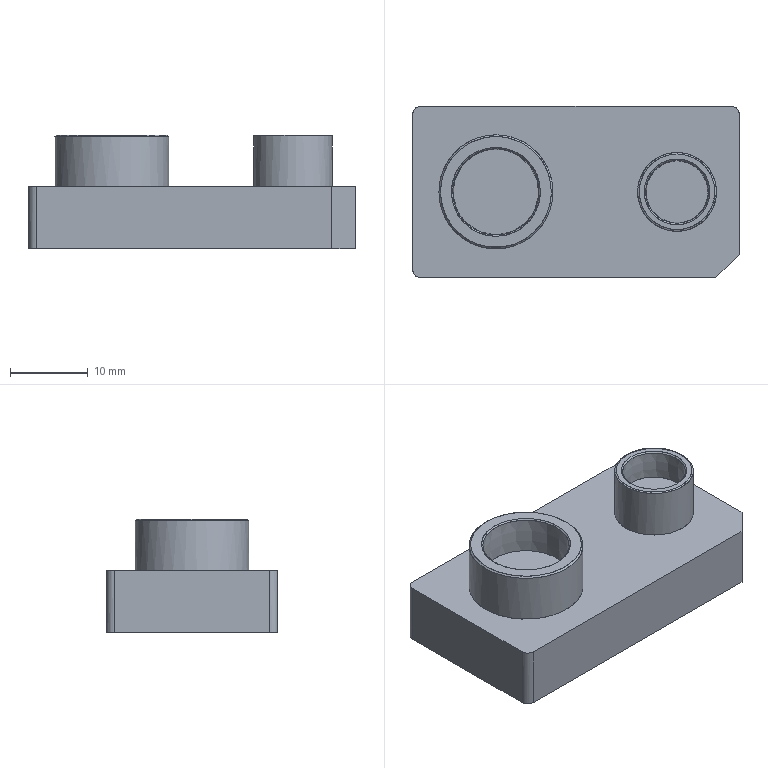NC program | PowerMill | posted by the shop | part box 42 x 22 x 14.621 mm
Lines 14234 to 15750 of 126517:
( TOOL ID   D4_2 )
( TOOL DIA. 4. TIP RAD 0 LENGTH 61.8 )
( Z = -6.79 )
T14 M6
T13
G91 G28 Z0
G0 G90 G54
M08
S18000 M3
X0 Y0 M8
G43 Z10.801 H14
X-9.103 Y-9.671
Z.911
G1 Z-.289 F1200
X-9.107 Y-9.621 F2000
X-9.116 Y-9.571
X-9.128 Y-9.522
X-9.144 Y-9.474
X-9.164 Y-9.428
X-9.187 Y-9.383
X-9.214 Y-9.34
X-9.244 Y-9.3
X-9.278 Y-9.262
X-9.314 Y-9.226
X-9.353 Y-9.194
X-9.394 Y-9.165
X-9.437 Y-9.139
X-9.483 Y-9.117
X-9.53 Y-9.098
X-9.578 Y-9.083
X-9.627 Y-9.072
X-9.677 Y-9.065
X-9.728 Y-9.062
X-9.773 Y-9.063
X-9.966 Y-9.072
X-10.153 Y-9.077
X-10.341 Y-9.078
X-10.531 Y-9.075
X-10.721 Y-9.069
X-10.911 Y-9.058
X-11.101 Y-9.043
X-11.292 Y-9.024
X-11.478 Y-9.002
X-11.665 Y-8.976
X-11.851 Y-8.945
X-12.039 Y-8.911
X-12.225 Y-8.873
X-12.412 Y-8.83
X-12.597 Y-8.784
X-12.781 Y-8.734
X-12.963 Y-8.68
X-13.139 Y-8.624
X-13.315 Y-8.564
X-13.493 Y-8.5
X-13.671 Y-8.431
X-13.847 Y-8.358
X-14.02 Y-8.283
X-14.188 Y-8.206
X-14.351 Y-8.126
X-14.519 Y-8.041
X-14.668 Y-7.961
X-14.833 Y-7.868
X-14.997 Y-7.771
X-15.158 Y-7.671
X-15.318 Y-7.568
X-15.469 Y-7.465
X-15.595 Y-7.377
X-15.719 Y-7.287
X-15.841 Y-7.195
X-15.961 Y-7.1
X-16.064 Y-7.017
X-16.166 Y-6.932
X-16.266 Y-6.846
X-16.365 Y-6.758
X-16.509 Y-6.627
X-16.618 Y-6.523
X-16.726 Y-6.417
X-16.832 Y-6.309
X-16.955 Y-6.179
X-17.057 Y-6.067
X-17.158 Y-5.954
X-17.256 Y-5.839
X-17.352 Y-5.723
X-17.472 Y-5.571
X-17.588 Y-5.418
X-17.701 Y-5.264
X-17.809 Y-5.108
X-17.914 Y-4.951
X-18.015 Y-4.792
X-18.113 Y-4.629
X-18.209 Y-4.464
X-18.301 Y-4.297
X-18.39 Y-4.127
X-18.476 Y-3.955
X-18.553 Y-3.791
X-18.627 Y-3.625
X-18.698 Y-3.458
X-18.768 Y-3.283
X-18.836 Y-3.103
X-18.899 Y-2.924
X-18.956 Y-2.751
X-19.009 Y-2.577
X-19.055 Y-2.416
X-19.098 Y-2.254
X-19.138 Y-2.091
X-19.176 Y-1.927
X-19.213 Y-1.748
X-19.246 Y-1.568
X-19.276 Y-1.388
X-19.302 Y-1.207
X-19.324 Y-1.026
X-19.344 Y-.837
X-19.359 Y-.649
X-19.371 Y-.46
X-19.378 Y-.285
X-19.382 Y-.11
Y.065
X-19.379 Y.24
X-19.373 Y.427
X-19.362 Y.616
X-19.347 Y.807
X-19.328 Y.997
X-19.305 Y1.185
X-19.279 Y1.37
X-19.248 Y1.556
X-19.214 Y1.742
X-19.175 Y1.929
X-19.132 Y2.116
X-19.087 Y2.3
X-19.038 Y2.479
X-18.985 Y2.658
X-18.928 Y2.837
X-18.866 Y3.018
X-18.8 Y3.198
X-18.731 Y3.377
X-18.659 Y3.552
X-18.584 Y3.724
X-18.505 Y3.894
X-18.423 Y4.063
X-18.336 Y4.231
X-18.246 Y4.398
X-18.152 Y4.564
X-18.053 Y4.729
X-17.951 Y4.892
X-17.848 Y5.05
X-17.741 Y5.206
X-17.631 Y5.361
X-17.517 Y5.513
X-17.399 Y5.664
X-17.278 Y5.812
X-17.174 Y5.936
X-17.067 Y6.057
X-16.957 Y6.176
X-16.839 Y6.301
X-16.726 Y6.417
X-16.611 Y6.53
X-16.494 Y6.641
X-16.361 Y6.762
X-16.246 Y6.864
X-16.129 Y6.963
X-16.011 Y7.06
X-15.891 Y7.156
X-15.753 Y7.261
X-15.61 Y7.367
X-15.457 Y7.474
X-15.299 Y7.58
X-15.148 Y7.678
X-15.001 Y7.769
X-14.846 Y7.861
X-14.689 Y7.949
X-14.526 Y8.037
X-14.355 Y8.124
X-14.189 Y8.205
X-14.026 Y8.28
X-13.861 Y8.353
X-13.695 Y8.421
X-13.519 Y8.49
X-13.341 Y8.555
X-13.162 Y8.617
X-12.982 Y8.674
X-12.801 Y8.728
X-12.62 Y8.778
X-12.438 Y8.824
X-12.252 Y8.867
X-12.066 Y8.906
X-11.879 Y8.941
X-11.692 Y8.972
X-11.505 Y8.999
X-11.317 Y9.022
X-11.127 Y9.041
X-10.936 Y9.056
X-10.746 Y9.067
X-10.555 Y9.075
X-10.365 Y9.078
X-10.174 Y9.077
X-9.984 Y9.073
X-9.794 Y9.064
X-9.604 Y9.051
X-9.414 Y9.034
X-9.225 Y9.014
X-9.036 Y8.989
X-8.847 Y8.96
X-8.659 Y8.928
X-8.473 Y8.892
X-8.288 Y8.851
X-8.103 Y8.807
X-7.919 Y8.759
X-7.735 Y8.707
X-7.552 Y8.651
X-7.377 Y8.593
X-7.203 Y8.532
X-7.026 Y8.465
X-6.865 Y8.401
X-6.706 Y8.334
X-6.542 Y8.262
X-6.385 Y8.189
X-6.23 Y8.112
X-6.072 Y8.031
X-5.916 Y7.947
X-5.761 Y7.86
X-5.609 Y7.77
X-5.458 Y7.676
X-5.311 Y7.581
X-5.171 Y7.487
X-5.033 Y7.391
X-4.898 Y7.293
X-4.764 Y7.191
X-4.634 Y7.09
X-4.506 Y6.985
X-4.369 Y6.869
X-4.237 Y6.752
X-4.106 Y6.633
X-3.978 Y6.511
X-3.853 Y6.387
X-3.73 Y6.26
X-3.617 Y6.139
X-3.505 Y6.015
X-3.396 Y5.889
X-3.289 Y5.762
X-3.185 Y5.633
X-3.084 Y5.502
X-2.985 Y5.37
X-2.888 Y5.236
X-2.794 Y5.1
X-2.702 Y4.962
X-2.6 Y4.801
X-2.502 Y4.64
X-2.408 Y4.479
X-2.318 Y4.316
X-2.229 Y4.147
X-2.144 Y3.978
X-2.064 Y3.808
X-1.988 Y3.64
X-1.917 Y3.474
X-1.846 Y3.296
X-1.778 Y3.118
X-1.715 Y2.938
X-1.655 Y2.757
X-1.599 Y2.575
X-1.551 Y2.406
X-1.506 Y2.235
X-1.464 Y2.064
X-1.423 Y1.877
X-1.388 Y1.705
X-1.356 Y1.531
X-1.328 Y1.357
X-1.302 Y1.168
X-1.279 Y.978
X-1.261 Y.787
X-1.246 Y.597
X-1.235 Y.406
X-1.229 Y.215
X-1.226 Y.024
X-1.228 Y-.167
X-1.233 Y-.352
X-1.242 Y-.538
X-1.255 Y-.727
X-1.273 Y-.918
X-1.294 Y-1.107
X-1.319 Y-1.292
X-1.347 Y-1.476
X-1.379 Y-1.66
X-1.416 Y-1.845
X-1.456 Y-2.031
X-1.501 Y-2.217
X-1.549 Y-2.399
X-1.601 Y-2.58
X-1.653 Y-2.752
X-1.709 Y-2.923
X-1.769 Y-3.093
X-1.832 Y-3.261
X-1.899 Y-3.428
X-1.968 Y-3.595
X-2.045 Y-3.768
X-2.121 Y-3.931
X-2.201 Y-4.092
X-2.283 Y-4.251
X-2.372 Y-4.415
X-2.468 Y-4.582
X-2.561 Y-4.739
X-2.656 Y-4.891
X-2.75 Y-5.035
X-2.846 Y-5.176
X-2.946 Y-5.316
X-3.047 Y-5.454
X-3.151 Y-5.59
X-3.258 Y-5.724
X-3.381 Y-5.872
X-3.507 Y-6.018
X-3.636 Y-6.16
X-3.768 Y-6.3
X-3.902 Y-6.436
X-4.026 Y-6.557
X-4.153 Y-6.676
X-4.285 Y-6.795
X-4.416 Y-6.909
X-4.549 Y-7.021
X-4.685 Y-7.13
X-4.83 Y-7.242
X-4.978 Y-7.352
X-5.129 Y-7.459
X-5.282 Y-7.562
X-5.436 Y-7.662
X-5.588 Y-7.757
X-5.742 Y-7.849
X-5.898 Y-7.937
X-6.056 Y-8.022
X-6.215 Y-8.105
X-6.376 Y-8.184
X-6.549 Y-8.265
X-6.699 Y-8.332
X-6.851 Y-8.396
X-7.004 Y-8.457
X-7.158 Y-8.515
X-7.313 Y-8.571
X-7.469 Y-8.624
X-7.644 Y-8.679
X-7.82 Y-8.732
X-7.999 Y-8.781
X-8.179 Y-8.826
X-8.358 Y-8.867
X-8.538 Y-8.905
X-8.719 Y-8.938
X-8.907 Y-8.97
X-9.095 Y-8.997
X-9.284 Y-9.021
X-9.472 Y-9.04
X-9.658 Y-9.055
X-9.773 Y-9.063
X-9.823 Y-9.068
X-9.873 Y-9.077
X-9.921 Y-9.09
X-9.969 Y-9.107
X-10.015 Y-9.128
X-10.06 Y-9.152
X-10.102 Y-9.179
X-10.142 Y-9.21
X-10.179 Y-9.244
X-10.214 Y-9.281
X-10.246 Y-9.32
X-10.274 Y-9.362
X-10.299 Y-9.406
X-10.321 Y-9.451
X-10.339 Y-9.499
X-10.353 Y-9.547
X-10.363 Y-9.597
X-10.369 Y-9.647
X-10.372 Y-9.697
X-10.37 Y-9.742
X-9.096 Y-9.684 Z-.309
X-9.101 Y-9.634
X-9.11 Y-9.584
X-9.122 Y-9.535
X-9.139 Y-9.488
X-9.159 Y-9.441
X-9.183 Y-9.397
X-9.21 Y-9.354
X-9.241 Y-9.314
X-9.275 Y-9.276
X-9.311 Y-9.241
X-9.35 Y-9.209
X-9.392 Y-9.181
X-9.436 Y-9.155
X-9.481 Y-9.133
X-9.528 Y-9.115
X-9.577 Y-9.101
X-9.626 Y-9.09
X-9.676 Y-9.084
X-9.727 Y-9.081
X-9.772 Y-9.082
X-9.88 Y-9.088
X-10.069 Y-9.095
X-10.258 Y-9.098
X-10.448 Y-9.097
X-10.638 Y-9.092
X-10.827 Y-9.083
X-11.017 Y-9.07
X-11.206 Y-9.053
X-11.396 Y-9.032
X-11.585 Y-9.008
X-11.774 Y-8.979
X-11.958 Y-8.947
X-12.143 Y-8.91
X-12.329 Y-8.87
X-12.516 Y-8.825
X-12.696 Y-8.778
X-12.877 Y-8.727
X-13.058 Y-8.671
X-13.241 Y-8.611
X-13.412 Y-8.551
X-13.582 Y-8.488
X-13.754 Y-8.419
X-13.929 Y-8.345
X-14.102 Y-8.267
X-14.274 Y-8.187
X-14.444 Y-8.102
X-14.612 Y-8.014
X-14.778 Y-7.922
X-14.943 Y-7.827
X-15.105 Y-7.728
X-15.266 Y-7.626
X-15.425 Y-7.52
X-15.574 Y-7.416
X-15.722 Y-7.309
X-15.867 Y-7.2
X-16.01 Y-7.087
X-16.151 Y-6.971
X-16.271 Y-6.869
X-16.387 Y-6.766
X-16.508 Y-6.655
X-16.624 Y-6.546
X-16.737 Y-6.434
X-16.848 Y-6.321
X-16.976 Y-6.186
X-17.083 Y-6.069
X-17.188 Y-5.949
X-17.291 Y-5.828
X-17.41 Y-5.682
X-17.512 Y-5.552
X-17.611 Y-5.421
X-17.709 Y-5.287
X-17.803 Y-5.152
X-17.895 Y-5.015
X-17.985 Y-4.877
X-18.082 Y-4.721
X-18.177 Y-4.561
X-18.269 Y-4.398
X-18.359 Y-4.231
X-18.446 Y-4.06
X-18.531 Y-3.885
X-18.608 Y-3.719
X-18.681 Y-3.55
X-18.753 Y-3.377
X-18.822 Y-3.199
X-18.887 Y-3.019
X-18.948 Y-2.841
X-19.004 Y-2.665
X-19.056 Y-2.489
X-19.104 Y-2.311
X-19.151 Y-2.126
X-19.193 Y-1.94
X-19.232 Y-1.754
X-19.267 Y-1.567
X-19.297 Y-1.38
X-19.324 Y-1.192
X-19.347 Y-1.004
X-19.366 Y-.815
X-19.381 Y-.626
X-19.392 Y-.436
X-19.399 Y-.246
X-19.402 Y-.055
Y.136
X-19.397 Y.326
X-19.388 Y.516
X-19.375 Y.706
X-19.358 Y.895
X-19.338 Y1.083
X-19.313 Y1.273
X-19.284 Y1.461
X-19.252 Y1.648
X-19.216 Y1.835
X-19.175 Y2.02
X-19.131 Y2.205
X-19.084 Y2.388
X-19.032 Y2.571
X-18.976 Y2.753
X-18.917 Y2.933
X-18.854 Y3.111
X-18.788 Y3.288
X-18.727 Y3.44
X-18.664 Y3.592
X-18.598 Y3.742
X-18.529 Y3.89
X-18.457 Y4.038
X-18.379 Y4.193
X-18.298 Y4.346
X-18.214 Y4.497
X-18.126 Y4.647
X-18.036 Y4.795
X-17.95 Y4.931
X-17.862 Y5.065
X-17.771 Y5.199
X-17.678 Y5.33
X-17.583 Y5.459
X-17.485 Y5.587
X-17.385 Y5.713
X-17.273 Y5.85
X-17.157 Y5.985
X-17.035 Y6.122
X-16.905 Y6.261
X-16.773 Y6.398
X-16.645 Y6.525
X-16.526 Y6.638
X-16.439 Y6.718
X-16.352 Y6.797
X-16.264 Y6.875
X-16.15 Y6.972
X-16.034 Y7.067
X-15.917 Y7.16
X-15.799 Y7.252
X-15.679 Y7.341
X-15.529 Y7.448
X-15.376 Y7.553
X-15.216 Y7.658
X-15.053 Y7.76
X-14.894 Y7.856
X-14.735 Y7.947
X-14.573 Y8.035
X-14.407 Y8.121
X-14.237 Y8.204
X-14.064 Y8.285
X-13.889 Y8.362
X-13.716 Y8.434
X-13.548 Y8.5
X-13.379 Y8.563
X-13.209 Y8.622
X-13.036 Y8.679
X-12.864 Y8.731
X-12.69 Y8.78
X-12.516 Y8.825
X-12.331 Y8.87
X-12.151 Y8.909
X-11.97 Y8.944
X-11.783 Y8.977
X-11.595 Y9.006
X-11.405 Y9.031
X-11.214 Y9.052
X-11.025 Y9.07
X-10.836 Y9.083
X-10.647 Y9.092
X-10.458 Y9.097
X-10.274 Y9.098
X-10.089 Y9.095
X-9.905 Y9.089
X-9.72 Y9.079
X-9.533 Y9.066
X-9.349 Y9.048
X-9.166 Y9.027
X-8.983 Y9.002
X-8.794 Y8.972
X-8.606 Y8.938
X-8.42 Y8.901
X-8.236 Y8.86
X-8.054 Y8.815
X-7.868 Y8.766
X-7.684 Y8.713
X-7.502 Y8.656
X-7.321 Y8.595
X-7.141 Y8.531
X-6.964 Y8.463
X-6.788 Y8.391
X-6.613 Y8.316
X-6.44 Y8.237
X-6.268 Y8.154
X-6.099 Y8.068
X-5.931 Y7.978
X-5.772 Y7.889
X-5.661 Y7.824
X-5.55 Y7.757
X-5.441 Y7.689
X-5.332 Y7.619
X-5.224 Y7.548
X-5.073 Y7.443
X-4.923 Y7.336
X-4.775 Y7.225
X-4.63 Y7.112
X-4.487 Y6.995
X-4.347 Y6.876
X-4.205 Y6.75
X-4.064 Y6.621
X-3.926 Y6.488
X-3.792 Y6.354
X-3.661 Y6.217
X-3.534 Y6.078
X-3.415 Y5.942
X-3.298 Y5.804
X-3.184 Y5.664
X-3.073 Y5.522
X-2.965 Y5.377
X-2.868 Y5.242
X-2.773 Y5.105
X-2.681 Y4.967
X-2.578 Y4.805
X-2.482 Y4.647
X-2.391 Y4.49
X-2.298 Y4.322
X-2.21 Y4.153
X-2.126 Y3.985
X-2.045 Y3.816
X-1.967 Y3.641
X-1.892 Y3.466
X-1.822 Y3.289
X-1.755 Y3.111
X-1.692 Y2.932
X-1.632 Y2.752
X-1.577 Y2.57
X-1.525 Y2.387
X-1.477 Y2.203
X-1.433 Y2.018
X-1.393 Y1.832
X-1.356 Y1.646
X-1.324 Y1.459
X-1.295 Y1.271
X-1.271 Y1.082
X-1.25 Y.895
X-1.234 Y.707
X-1.221 Y.519
X-1.212 Y.33
X-1.207 Y.141
X-1.206 Y-.049
X-1.209 Y-.238
X-1.216 Y-.427
X-1.227 Y-.617
X-1.242 Y-.807
X-1.261 Y-.997
X-1.284 Y-1.187
X-1.311 Y-1.376
X-1.341 Y-1.562
X-1.376 Y-1.749
X-1.414 Y-1.935
X-1.457 Y-2.122
X-1.504 Y-2.308
X-1.551 Y-2.482
X-1.6 Y-2.649
X-1.653 Y-2.814
X-1.709 Y-2.983
X-1.771 Y-3.155
X-1.833 Y-3.318
X-1.897 Y-3.479
X-1.966 Y-3.638
X-2.044 Y-3.813
X-2.122 Y-3.977
X-2.203 Y-4.141
X-2.292 Y-4.31
X-2.384 Y-4.477
X-2.48 Y-4.642
X-2.578 Y-4.805
X-2.68 Y-4.965
X-2.785 Y-5.122
X-2.89 Y-5.273
X-2.998 Y-5.422
X-3.109 Y-5.568
X-3.223 Y-5.712
X-3.34 Y-5.854
X-3.459 Y-5.993
X-3.585 Y-6.134
X-3.714 Y-6.272
X-3.846 Y-6.408
X-3.982 Y-6.542
X-4.12 Y-6.673
X-4.26 Y-6.8
X-4.403 Y-6.925
X-4.547 Y-7.045
X-4.693 Y-7.162
X-4.843 Y-7.276
X-4.996 Y-7.389
X-5.152 Y-7.498
X-5.312 Y-7.606
X-5.473 Y-7.709
X-5.636 Y-7.809
X-5.787 Y-7.898
X-5.94 Y-7.983
X-6.095 Y-8.066
X-6.259 Y-8.149
X-6.416 Y-8.225
X-6.575 Y-8.299
X-6.736 Y-8.369
X-6.904 Y-8.439
X-7.074 Y-8.505
X-7.253 Y-8.571
X-7.426 Y-8.631
X-7.599 Y-8.687
X-7.774 Y-8.739
X-7.959 Y-8.791
X-8.144 Y-8.838
X-8.328 Y-8.881
X-8.512 Y-8.92
X-8.693 Y-8.954
X-8.874 Y-8.985
X-9.062 Y-9.013
X-9.245 Y-9.036
X-9.428 Y-9.056
X-9.498 Y-9.062
X-9.689 Y-9.077
X-9.772 Y-9.082
X-9.822 Y-9.087
X-9.872 Y-9.096
X-9.921 Y-9.108
X-9.968 Y-9.125
X-10.015 Y-9.145
X-10.059 Y-9.169
X-10.102 Y-9.196
X-10.142 Y-9.227
X-10.18 Y-9.261
X-10.215 Y-9.297
X-10.246 Y-9.336
X-10.275 Y-9.378
X-10.301 Y-9.422
X-10.322 Y-9.467
X-10.341 Y-9.514
X-10.355 Y-9.563
X-10.366 Y-9.612
X-10.372 Y-9.662
X-10.375 Y-9.713
X-10.374 Y-9.758
X-9.094 Y-9.704 Z-.329
X-9.099 Y-9.653
X-9.108 Y-9.604
X-9.121 Y-9.555
X-9.137 Y-9.507
X-9.158 Y-9.461
X-9.182 Y-9.416
X-9.209 Y-9.374
X-9.24 Y-9.333
X-9.273 Y-9.296
X-9.31 Y-9.261
X-9.349 Y-9.229
X-9.391 Y-9.2
X-9.434 Y-9.175
X-9.48 Y-9.153
X-9.527 Y-9.135
X-9.576 Y-9.121
X-9.625 Y-9.11
X-9.675 Y-9.104
X-9.725 Y-9.101
X-9.77 Y-9.102
X-9.869 Y-9.108
X-10.06 Y-9.115
X-10.251 Y-9.118
X-10.441 Y-9.117
X-10.631 Y-9.112
X-10.821 Y-9.104
X-11.009 Y-9.091
X-11.198 Y-9.074
X-11.387 Y-9.053
X-11.576 Y-9.029
X-11.764 Y-9.
X-11.951 Y-8.968
X-12.138 Y-8.932
X-12.324 Y-8.892
X-12.508 Y-8.848
X-12.684 Y-8.802
X-12.859 Y-8.753
X-13.033 Y-8.7
X-13.215 Y-8.641
X-13.391 Y-8.58
X-13.562 Y-8.517
X-13.731 Y-8.45
X-13.898 Y-8.38
X-14.074 Y-8.302
X-14.247 Y-8.221
X-14.419 Y-8.137
X-14.589 Y-8.049
X-14.756 Y-7.958
X-14.921 Y-7.863
X-15.084 Y-7.765
X-15.242 Y-7.665
X-15.401 Y-7.561
X-15.559 Y-7.451
X-15.714 Y-7.34
X-15.867 Y-7.225
X-16.016 Y-7.108
X-16.163 Y-6.987
X-16.301 Y-6.869
X-16.434 Y-6.75
X-16.573 Y-6.621
X-16.709 Y-6.49
X-16.843 Y-6.355
X-16.975 Y-6.216
X-17.102 Y-6.078
X-17.225 Y-5.937
X-17.346 Y-5.793
X-17.464 Y-5.646
X-17.583 Y-5.492
X-17.695 Y-5.341
X-17.8 Y-5.192
X-17.894 Y-5.054
X-18.003 Y-4.885
X-18.1 Y-4.73
X-18.186 Y-4.585
X-18.26 Y-4.455
X-18.333 Y-4.324
X-18.402 Y-4.192
X-18.469 Y-4.058
X-18.535 Y-3.923
X-18.611 Y-3.761
X-18.685 Y-3.593
X-18.755 Y-3.424
X-18.821 Y-3.258
X-18.888 Y-3.076
X-18.951 Y-2.895
X-19.009 Y-2.714
X-19.064 Y-2.533
X-19.114 Y-2.351
X-19.162 Y-2.166
X-19.205 Y-1.98
X-19.244 Y-1.794
X-19.28 Y-1.607
X-19.311 Y-1.42
X-19.338 Y-1.24
X-19.361 Y-1.059
X-19.38 Y-.878
X-19.396 Y-.695
X-19.408 Y-.514
X-19.416 Y-.332
X-19.421 Y-.149
X-19.422 Y.035
X-19.42 Y.219
X-19.414 Y.406
X-19.404 Y.591
X-19.39 Y.774
X-19.372 Y.957
X-19.351 Y1.136
X-19.327 Y1.315
X-19.3 Y1.493
X-19.268 Y1.671
X-19.233 Y1.847
X-19.195 Y2.023
X-19.151 Y2.208
X-19.103 Y2.392
X-19.052 Y2.574
X-18.997 Y2.754
X-18.937 Y2.936
X-18.873 Y3.117
X-18.814 Y3.276
X-18.752 Y3.433
X-18.686 Y3.589
X-18.613 Y3.755
X-18.542 Y3.909
X-18.468 Y4.061
X-18.391 Y4.212
X-18.3 Y4.382
X-18.21 Y4.543
X-18.117 Y4.702
X-18.019 Y4.861
X-17.916 Y5.02
X-17.808 Y5.18
X-17.695 Y5.34
X-17.592 Y5.48
X-17.48 Y5.625
X-17.357 Y5.779
X-17.253 Y5.905
X-17.146 Y6.028
X-17.036 Y6.15
X-16.913 Y6.282
X-16.8 Y6.399
X-16.684 Y6.515
X-16.566 Y6.628
X-16.446 Y6.739
X-16.302 Y6.868
X-16.156 Y6.992
X-16.011 Y7.112
X-15.865 Y7.227
X-15.726 Y7.331
X-15.59 Y7.43
X-15.452 Y7.526
X-15.312 Y7.62
X-15.17 Y7.711
X-15.026 Y7.8
X-14.875 Y7.89
X-14.721 Y7.978
X-14.565 Y8.062
X-14.408 Y8.143
X-14.249 Y8.22
X-14.093 Y8.294
X-13.936 Y8.364
X-13.768 Y8.435
X-13.608 Y8.499
X-13.447 Y8.56
X-13.265 Y8.624
X-13.083 Y8.684
X-12.899 Y8.741
X-12.715 Y8.794
X-12.53 Y8.842
X-12.344 Y8.887
X-12.158 Y8.928
X-11.972 Y8.964
X-11.785 Y8.997
X-11.597 Y9.026
X-11.407 Y9.051
X-11.216 Y9.072
X-11.031 Y9.089
X-10.846 Y9.102
X-10.659 Y9.111
X-10.469 Y9.117
X-10.277 Y9.118
X-10.088 Y9.116
X-9.902 Y9.109
X-9.717 Y9.099
X-9.526 Y9.085
X-9.336 Y9.067
X-9.146 Y9.044
X-8.957 Y9.018
X-8.768 Y8.988
X-8.579 Y8.954
X-8.395 Y8.916
X-8.21 Y8.874
X-8.026 Y8.829
X-7.841 Y8.779
X-7.655 Y8.725
X-7.483 Y8.671
X-7.311 Y8.613
X-7.14 Y8.552
X-6.967 Y8.485
X-6.789 Y8.413
X-6.614 Y8.338
X-6.446 Y8.262
X-6.283 Y8.183
X-6.121 Y8.102
X-5.961 Y8.017
X-5.793 Y7.924
X-5.628 Y7.828
X-5.467 Y7.729
X-5.308 Y7.628
X-5.153 Y7.523
X-5. Y7.416
X-4.851 Y7.307
X-4.705 Y7.196
X-4.561 Y7.082
X-4.419 Y6.965
X-4.28 Y6.844
X-4.167 Y6.743
X-4.053 Y6.638
X-3.933 Y6.522
X-3.815 Y6.406
X-3.698 Y6.285
X-3.573 Y6.151
X-3.457 Y6.021
X-3.348 Y5.895
X-3.235 Y5.759
X-3.124 Y5.621
X-3.016 Y5.48
X-2.911 Y5.338
X-2.806 Y5.188
X-2.699 Y5.03
X-2.597 Y4.872
X-2.498 Y4.711
X-2.401 Y4.548
X-2.309 Y4.384
X-2.218 Y4.214
X-2.134 Y4.048
X-2.054 Y3.884
X-1.977 Y3.714
X-1.9 Y3.535
X-1.828 Y3.361
X-1.76 Y3.185
X-1.696 Y3.006
X-1.635 Y2.826
X-1.578 Y2.643
X-1.525 Y2.46
X-1.475 Y2.276
X-1.429 Y2.092
X-1.388 Y1.906
X-1.35 Y1.72
X-1.316 Y1.532
X-1.286 Y1.344
X-1.26 Y1.155
X-1.238 Y.968
X-1.22 Y.781
X-1.206 Y.593
X-1.195 Y.404
X-1.189 Y.214
X-1.186 Y.025
X-1.188 Y-.164
X-1.193 Y-.353
X-1.202 Y-.543
X-1.216 Y-.733
X-1.233 Y-.923
X-1.254 Y-1.113
X-1.28 Y-1.302
X-1.309 Y-1.49
X-1.342 Y-1.677
X-1.379 Y-1.864
X-1.42 Y-2.051
X-1.465 Y-2.236
X-1.514 Y-2.421
X-1.566 Y-2.605
X-1.622 Y-2.786
X-1.682 Y-2.967
X-1.746 Y-3.146
X-1.813 Y-3.323
X-1.884 Y-3.499
X-1.959 Y-3.674
X-2.038 Y-3.848
X-2.115 Y-4.008
X-2.194 Y-4.166
X-2.276 Y-4.323
X-2.362 Y-4.479
X-2.45 Y-4.632
X-2.542 Y-4.784
X-2.637 Y-4.933
X-2.743 Y-5.095
X-2.85 Y-5.251
X-2.944 Y-5.383
X-3.041 Y-5.512
X-3.14 Y-5.64
X-3.247 Y-5.773
X-3.35 Y-5.897
X-3.455 Y-6.019
X-3.549 Y-6.124
X-3.645 Y-6.228
X-3.742 Y-6.33
X-3.84 Y-6.431
X-3.941 Y-6.53
X-4.059 Y-6.643
X-4.178 Y-6.754
X-4.3 Y-6.862
X-4.424 Y-6.968
X-4.549 Y-7.072
X-4.697 Y-7.19
X-4.847 Y-7.305
X-5.001 Y-7.417
X-5.158 Y-7.527
X-5.314 Y-7.631
X-5.474 Y-7.733
X-5.636 Y-7.832
X-5.802 Y-7.929
X-5.971 Y-8.022
X-6.137 Y-8.11
X-6.305 Y-8.194
X-6.475 Y-8.275
X-6.649 Y-8.353
X-6.822 Y-8.427
X-6.997 Y-8.497
X-7.174 Y-8.564
X-7.352 Y-8.627
X-7.532 Y-8.686
X-7.718 Y-8.743
X-7.904 Y-8.796
X-8.088 Y-8.845
X-8.272 Y-8.889
X-8.456 Y-8.929
X-8.625 Y-8.962
X-8.795 Y-8.992
X-8.965 Y-9.019
X-9.136 Y-9.043
X-9.298 Y-9.062
X-9.488 Y-9.081
X-9.679 Y-9.097
X-9.77 Y-9.102
X-9.821 Y-9.107
X-9.87 Y-9.116
X-9.919 Y-9.129
X-9.967 Y-9.145
X-10.013 Y-9.166
X-10.058 Y-9.189
X-10.1 Y-9.217
X-10.141 Y-9.247
X-10.178 Y-9.281
X-10.213 Y-9.318
X-10.245 Y-9.357
X-10.274 Y-9.398
X-10.299 Y-9.442
X-10.321 Y-9.488
X-10.339 Y-9.535
X-10.353 Y-9.583
X-10.364 Y-9.633
X-10.37 Y-9.683
X-10.373 Y-9.733
X-10.372 Y-9.778
X-9.092 Y-9.723 Z-.349
X-9.097 Y-9.672
X-9.106 Y-9.623
X-9.119 Y-9.574
X-9.136 Y-9.526
X-9.156 Y-9.48
X-9.18 Y-9.435
X-9.208 Y-9.393
X-9.238 Y-9.353
X-9.272 Y-9.315
X-9.308 Y-9.28
X-9.348 Y-9.248
X-9.389 Y-9.22
X-9.433 Y-9.194
X-9.479 Y-9.173
X-9.526 Y-9.155
X-9.574 Y-9.14
X-9.624 Y-9.13
X-9.674 Y-9.123
X-9.724 Y-9.121
X-9.769 Y-9.122
X-9.858 Y-9.127
X-10.038 Y-9.134
X-10.219 Y-9.138
X-10.399
X-10.579 Y-9.134
X-10.765 Y-9.127
X-10.945 Y-9.116
X-11.124 Y-9.101
X-11.316 Y-9.082
X-11.506 Y-9.059
X-11.696 Y-9.032
X-11.885 Y-9.
X-12.073 Y-8.965
X-12.258 Y-8.927
X-12.442 Y-8.885
X-12.626 Y-8.838
X-12.81 Y-8.788
X-12.994 Y-8.733
X-13.177 Y-8.675
X-13.358 Y-8.613
X-13.538 Y-8.547
X-13.716 Y-8.478
X-13.887 Y-8.407
X-14.058 Y-8.332
X-14.23 Y-8.252
X-14.402 Y-8.168
X-14.573 Y-8.08
X-14.741 Y-7.989
X-14.906 Y-7.895
X-15.066 Y-7.8
X-15.223 Y-7.701
X-15.375 Y-7.602
X-15.524 Y-7.501
X-15.672 Y-7.396
X-15.817 Y-7.288
X-15.968 Y-7.171
X-16.117 Y-7.051
X-16.263 Y-6.928
X-16.406 Y-6.802
X-16.547 Y-6.674
X-16.678 Y-6.548
X-16.807 Y-6.42
X-16.939 Y-6.284
X-17.068 Y-6.145
X-17.188 Y-6.01
X-17.306 Y-5.872
X-17.421 Y-5.732
X-17.529 Y-5.595
X-17.635 Y-5.456
X-17.738 Y-5.316
X-17.838 Y-5.173
X-17.935 Y-5.028
X-18.029 Y-4.882
X-18.129 Y-4.72
X-18.226 Y-4.556
X-18.319 Y-4.39
X-18.409 Y-4.221
X-18.494 Y-4.054
X-18.576 Y-3.885
X-18.654 Y-3.714
X-18.729 Y-3.54
X-18.801 Y-3.364
X-18.869 Y-3.187
X-18.933 Y-3.01
X-18.993 Y-2.829
X-19.051 Y-2.648
X-19.104 Y-2.465
X-19.154 Y-2.28
X-19.197 Y-2.106
X-19.236 Y-1.931
X-19.272 Y-1.756
X-19.306 Y-1.57
X-19.336 Y-1.392
X-19.362 Y-1.215
X-19.384 Y-1.037
X-19.403 Y-.855
X-19.418 Y-.672
X-19.43 Y-.482
X-19.438 Y-.29
X-19.442 Y-.104
Y.08
X-19.439 Y.263
X-19.431 Y.454
X-19.42 Y.644
X-19.404 Y.834
X-19.385 Y1.024
X-19.362 Y1.214
X-19.334 Y1.403
X-19.305 Y1.58
X-19.272 Y1.758
X-19.236 Y1.934
X-19.196 Y2.11
X-19.152 Y2.285
X-19.105 Y2.459
X-19.058 Y2.621
X-19.009 Y2.783
X-18.956 Y2.944
X-18.9 Y3.103
X-18.84 Y3.262
X-18.778 Y3.419
X-18.709 Y3.587
X-18.637 Y3.753
X-18.561 Y3.917
X-18.479 Y4.085
X-18.396 Y4.247
X-18.31 Y4.406
X-18.222 Y4.563
X-18.13 Y4.719
X-18.033 Y4.876
X-17.93 Y5.036
X-17.826 Y5.189
X-17.719 Y5.341
X-17.607 Y5.494
X-17.495 Y5.639
X-17.381 Y5.782
X-17.264 Y5.922
X-17.142 Y6.063
X-17.019 Y6.199
X-16.893 Y6.332
X-16.766 Y6.462
X-16.636 Y6.589
X-16.503 Y6.715
X-16.366 Y6.838
X-16.229 Y6.958
X-16.089 Y7.075
X-15.946 Y7.188
X-15.793 Y7.306
X-15.639 Y7.419
X-15.484 Y7.529
X-15.327 Y7.634
X-15.169 Y7.736
X-15.005 Y7.836
X-14.84 Y7.933
X-14.672 Y8.027
X-14.503 Y8.117
X-14.331 Y8.203
X-14.161 Y8.285
X-13.988 Y8.363
X-13.813 Y8.438
X-13.637 Y8.509
X-13.458 Y8.577
X-13.278 Y8.641
X-13.096 Y8.701
X-12.93 Y8.753
X-12.763 Y8.801
X-12.595 Y8.847
X-12.426 Y8.888
X-12.256 Y8.927
X-12.086 Y8.963
X-11.899 Y8.998
X-11.712 Y9.029
X-11.524 Y9.056
X-11.334 Y9.08
X-11.143 Y9.1
X-10.958 Y9.115
X-10.772 Y9.126
X-10.584 Y9.134
X-10.392 Y9.138
X-10.2 Y9.137
X-10.013 Y9.134
X-9.827 Y9.126
X-9.641 Y9.114
X-9.452 Y9.098
X-9.262 Y9.079
X-9.073 Y9.055
X-8.884 Y9.027
X-8.698 Y8.996
X-8.517 Y8.962
X-8.33 Y8.922
X-8.144 Y8.879
X-7.958 Y8.832
X-7.774 Y8.781
X-7.591 Y8.726
X-7.409 Y8.667
X-7.229 Y8.605
X-7.049 Y8.539
X-6.871 Y8.469
X-6.695 Y8.395
X-6.52 Y8.318
X-6.347 Y8.237
X-6.176 Y8.152
X-6.007 Y8.065
X-5.84 Y7.973
X-5.675 Y7.879
X-5.516 Y7.783
X-5.358 Y7.684
X-5.202 Y7.581
X-5.047 Y7.475
X-4.894 Y7.364
X-4.743 Y7.251
X-4.596 Y7.136
X-4.452 Y7.018
X-4.324 Y6.91
X-4.199 Y6.799
X-4.075 Y6.686
X-3.954 Y6.571
X-3.835 Y6.454
X-3.71 Y6.326
X-3.583 Y6.191
X-3.455 Y6.049
X-3.331 Y5.906
X-3.211 Y5.761
X-3.093 Y5.613
X-2.98 Y5.464
X-2.876 Y5.322
X-2.775 Y5.178
X-2.677 Y5.033
X-2.582 Y4.885
X-2.483 Y4.725
X-2.386 Y4.56
X-2.292 Y4.394
X-2.202 Y4.226
X-2.116 Y4.056
X-2.033 Y3.884
X-1.953 Y3.711
X-1.878 Y3.535
X-1.805 Y3.358
X-1.737 Y3.179
X-1.672 Y2.998
X-1.613 Y2.821
X-1.557 Y2.643
X-1.504 Y2.46
X-1.454 Y2.275
X-1.408 Y2.089
X-1.367 Y1.903
X-1.329 Y1.72
X-1.296 Y1.536
X-1.266 Y1.349
X-1.24 Y1.161
X-1.218 Y.972
X-1.2 Y.783
X-1.186 Y.594
X-1.175 Y.406
X-1.169 Y.232
X-1.166 Y.058
X-1.167 Y-.116
X-1.171 Y-.29
X-1.178 Y-.471
X-1.19 Y-.654
X-1.205 Y-.843
X-1.225 Y-1.034
X-1.249 Y-1.224
X-1.276 Y-1.409
X-1.305 Y-1.588
X-1.337 Y-1.761
X-1.373 Y-1.933
X-1.412 Y-2.104
X-1.457 Y-2.287
X-1.506 Y-2.47
X-1.555 Y-2.639
X-1.608 Y-2.807
X-1.664 Y-2.974
X-1.73 Y-3.159
X-1.798 Y-3.338
X-1.867 Y-3.509
X-1.938 Y-3.675
X-2.018 Y-3.853
X-2.101 Y-4.027
X-2.187 Y-4.197
X-2.275 Y-4.363
X-2.366 Y-4.526
X-2.459 Y-4.687
X-2.558 Y-4.847
X-2.655 Y-4.999
X-2.749 Y-5.141
X-2.846 Y-5.281
X-2.946 Y-5.419
X-3.06 Y-5.57
X-3.177 Y-5.719
X-3.297 Y-5.866
X-3.405 Y-5.991
X-3.514 Y-6.115
X-3.626 Y-6.237
X-3.739 Y-6.357
X-3.855 Y-6.474
X-3.973 Y-6.59
X-4.107 Y-6.715
X-4.242 Y-6.838
X-4.381 Y-6.959
X-4.521 Y-7.076
X-4.664 Y-7.19
X-4.809 Y-7.301
X-4.963 Y-7.414
X-5.12 Y-7.525
X-5.28 Y-7.633
X-5.437 Y-7.734
X-5.595 Y-7.831
X-5.758 Y-7.927
X-5.925 Y-8.021
X-6.095 Y-8.111
X-6.265 Y-8.197
X-6.435 Y-8.279
X-6.605 Y-8.356
X-6.764 Y-8.424
X-6.924 Y-8.49
X-7.086 Y-8.553
X-7.248 Y-8.612
X-7.429 Y-8.674
X-7.612 Y-8.732
X-7.795 Y-8.787
X-7.98 Y-8.838
X-8.166 Y-8.885
X-8.354 Y-8.928
X-8.542 Y-8.967
X-8.676 Y-8.992
X-8.81 Y-9.015
X-8.945 Y-9.036
X-9.08 Y-9.056
X-9.131 Y-9.063
X-9.311 Y-9.084
X-9.491 Y-9.102
X-9.677 Y-9.116
X-9.769 Y-9.122
X-9.82 Y-9.127
X-9.869 Y-9.136
X-9.918 Y-9.149
X-9.966 Y-9.165
X-10.012 Y-9.186
X-10.057 Y-9.21
X-10.099 Y-9.237
X-10.139 Y-9.268
X-10.177 Y-9.301
X-10.212 Y-9.338
X-10.244 Y-9.377
X-10.272 Y-9.419
X-10.298 Y-9.462
X-10.319 Y-9.508
X-10.337 Y-9.555
X-10.352 Y-9.604
X-10.362 Y-9.653
X-10.369 Y-9.703
X-10.371 Y-9.754
X-10.37 Y-9.799
X-9.095 Y-9.748 Z-.369
X-9.1 Y-9.697
X-9.109 Y-9.647
X-9.121 Y-9.599
X-9.138 Y-9.551
X-9.158 Y-9.504
X-9.181 Y-9.46
X-9.208 Y-9.417
X-9.239 Y-9.377
X-9.272 Y-9.339
X-9.309 Y-9.304
X-9.347 Y-9.272
X-9.389 Y-9.243
X-9.432 Y-9.217
X-9.478 Y-9.195
X-9.525 Y-9.176
X-9.573 Y-9.162
X-9.623 Y-9.151
X-9.673 Y-9.144
X-9.723 Y-9.141
X-9.768 Y-9.142
X-9.918 Y-9.15
X-10.111 Y-9.156
X-10.29 Y-9.158
X-10.468 Y-9.157
X-10.65 Y-9.152
X-10.828 Y-9.143
X-11.006 Y-9.131
X-11.184 Y-9.116
X-11.374 Y-9.095
X-11.564 Y-9.071
X-11.753 Y-9.043
X-11.942 Y-9.01
X-12.131 Y-8.974
X-12.319 Y-8.934
X-12.506 Y-8.89
X-12.692 Y-8.842
X-12.869 Y-8.792
X-13.044 Y-8.739
X-13.222 Y-8.681
X-13.404 Y-8.618
X-13.582 Y-8.551
X-13.753 Y-8.484
X-13.922 Y-8.414
X-14.073 Y-8.347
X-14.224 Y-8.277
X-14.373 Y-8.204
X-14.535 Y-8.122
X-14.682 Y-8.044
X-14.827 Y-7.964
X-14.97 Y-7.88
X-15.126 Y-7.786
X-15.28 Y-7.688
X-15.432 Y-7.588
X-15.582 Y-7.484
X-15.73 Y-7.378
X-15.885 Y-7.262
X-16.036 Y-7.143
X-16.184 Y-7.022
X-16.329 Y-6.898
X-16.47 Y-6.772
X-16.609 Y-6.643
X-16.724 Y-6.532
X-16.848 Y-6.407
X-16.933 Y-6.32
X-17.017 Y-6.231
X-17.099 Y-6.14
X-17.18 Y-6.049
X-17.26 Y-5.957
X-17.339 Y-5.864
X-17.421 Y-5.764
X-17.502 Y-5.662
X-17.582 Y-5.559
X-17.66 Y-5.456
X-17.737 Y-5.351
X-17.843 Y-5.201
X-17.945 Y-5.049
X-18.044 Y-4.895
X-18.141 Y-4.74
X-18.239 Y-4.574
X-18.333 Y-4.407
X-18.423 Y-4.238
X-18.505 Y-4.078